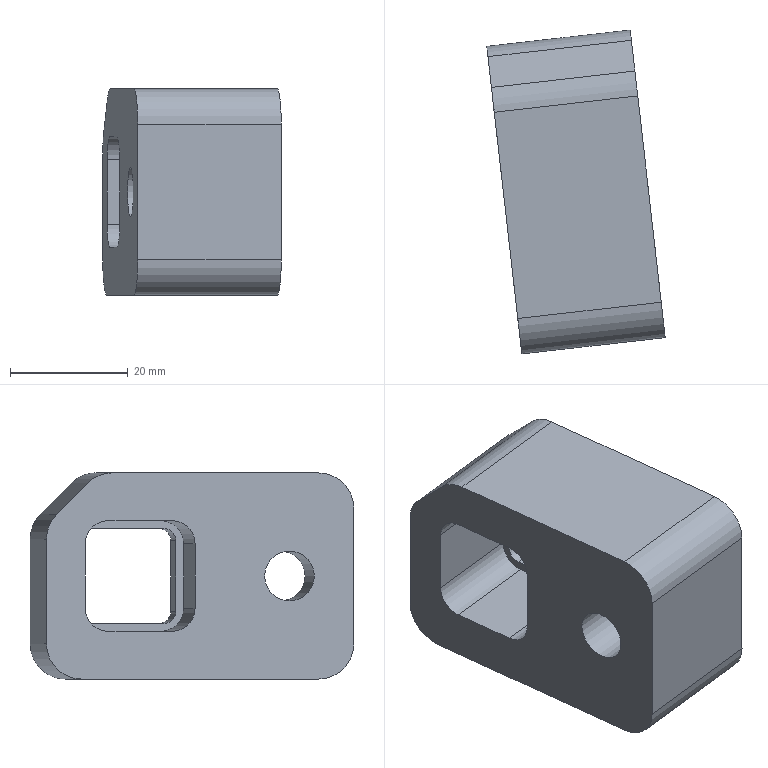Part | NX | features solid 2 | 1 solid | 32 faces | box 30.286 x 54.936 x 35 mm | volume 33387 mm3 | plane 17 | cylinder 15 | commonest cylinder face diameters 12 x5 4.08 x4 7.75 x4 8.5 x1 14 x1
STEP:
#1=CARTESIAN_POINT('',(3191.515,360.034,-76.987));
#2=VERTEX_POINT('',#1);
#3=CARTESIAN_POINT('',(3191.076,363.884,-80.862));
#4=VERTEX_POINT('',#3);
#5=CARTESIAN_POINT('',(3191.515,360.034,-80.862));
#6=DIRECTION('',(-0.9936,-0.1132,-0.000000001));
#7=DIRECTION('',(0.000000001,0.,-1.));
#8=AXIS2_PLACEMENT_3D('',#5,#6,#7);
#9=CIRCLE('',#8,3.875);
#10=EDGE_CURVE('',#2,#4,#9,.T.);
#11=ORIENTED_EDGE('',*,*,#10,.T.);
#12=CARTESIAN_POINT('',(3191.076,363.884,-91.862));
#13=VERTEX_POINT('',#12);
#14=CARTESIAN_POINT('',(3191.076,363.884,-86.362));
#15=DIRECTION('',(0.000000001,0.,-1.));
#16=VECTOR('',#15,1000.);
#17=LINE('',#14,#16);
#18=EDGE_CURVE('',#4,#13,#17,.T.);
#19=ORIENTED_EDGE('',*,*,#18,.T.);
#20=CARTESIAN_POINT('',(3191.515,360.034,-95.737));
#21=VERTEX_POINT('',#20);
#22=CARTESIAN_POINT('',(3191.515,360.034,-91.862));
#23=DIRECTION('',(-0.9936,-0.1132,-0.000000001));
#24=DIRECTION('',(0.000000001,0.,-1.));
#25=AXIS2_PLACEMENT_3D('',#22,#23,#24);
#26=CIRCLE('',#25,3.875);
#27=EDGE_CURVE('',#13,#21,#26,.T.);
#28=ORIENTED_EDGE('',*,*,#27,.T.);
#29=CARTESIAN_POINT('',(3192.76,349.105,-95.737));
#30=VERTEX_POINT('',#29);
#31=CARTESIAN_POINT('',(3192.222,353.824,-95.737));
#32=DIRECTION('',(0.1132,-0.9936,0.));
#33=VECTOR('',#32,1000.);
#34=LINE('',#31,#33);
#35=EDGE_CURVE('',#21,#30,#34,.T.);
#36=ORIENTED_EDGE('',*,*,#35,.T.);
#37=CARTESIAN_POINT('',(3193.198,345.255,-91.862));
#38=VERTEX_POINT('',#37);
#39=CARTESIAN_POINT('',(3192.76,349.105,-91.862));
#40=DIRECTION('',(0.9936,0.1132,0.000000001));
#41=DIRECTION('',(0.000000001,0.,-1.));
#42=AXIS2_PLACEMENT_3D('',#39,#40,#41);
#43=CIRCLE('',#42,3.875);
#44=EDGE_CURVE('',#38,#30,#43,.T.);
#45=ORIENTED_EDGE('',*,*,#44,.F.);
#46=CARTESIAN_POINT('',(3193.198,345.255,-80.862));
#47=VERTEX_POINT('',#46);
#48=CARTESIAN_POINT('',(3193.198,345.255,-91.862));
#49=DIRECTION('',(0.000000001,0.,-1.));
#50=VECTOR('',#49,1000.);
#51=LINE('',#48,#50);
#52=EDGE_CURVE('',#47,#38,#51,.T.);
#53=ORIENTED_EDGE('',*,*,#52,.F.);
#54=CARTESIAN_POINT('',(3192.76,349.105,-76.987));
#55=VERTEX_POINT('',#54);
#56=CARTESIAN_POINT('',(3192.76,349.105,-80.862));
#57=DIRECTION('',(0.9936,0.1132,0.000000001));
#58=DIRECTION('',(0.000000001,0.,-1.));
#59=AXIS2_PLACEMENT_3D('',#56,#57,#58);
#60=CIRCLE('',#59,3.875);
#61=EDGE_CURVE('',#55,#47,#60,.T.);
#62=ORIENTED_EDGE('',*,*,#61,.F.);
#63=CARTESIAN_POINT('',(3192.76,349.105,-76.987));
#64=DIRECTION('',(0.1132,-0.9936,0.));
#65=VECTOR('',#64,1000.);
#66=LINE('',#63,#65);
#67=EDGE_CURVE('',#2,#55,#66,.T.);
#68=ORIENTED_EDGE('',*,*,#67,.F.);
#69=EDGE_LOOP('',(#11,#19,#28,#36,#45,#53,#62,#68));
#70=FACE_BOUND('',#69,.T.);
#71=CARTESIAN_POINT('',(3193.047,346.581,-80.362));
#72=VERTEX_POINT('',#71);
#73=CARTESIAN_POINT('',(3193.047,346.581,-92.362));
#74=VERTEX_POINT('',#73);
#75=CARTESIAN_POINT('',(3193.047,346.581,-86.362));
#76=DIRECTION('',(0.000000001,-0.000000001,-1.));
#77=VECTOR('',#76,1000.);
#78=LINE('',#75,#77);
#79=EDGE_CURVE('',#72,#74,#78,.T.);
#80=ORIENTED_EDGE('',*,*,#79,.T.);
#81=CARTESIAN_POINT('',(3192.816,348.608,-94.402));
#82=VERTEX_POINT('',#81);
#83=CARTESIAN_POINT('',(3192.816,348.608,-92.362));
#84=DIRECTION('',(0.9936,0.1132,0.000000001));
#85=DIRECTION('',(0.000000001,0.,-1.));
#86=AXIS2_PLACEMENT_3D('',#83,#84,#85);
#87=CIRCLE('',#86,2.04);
#88=EDGE_CURVE('',#74,#82,#87,.T.);
#89=ORIENTED_EDGE('',*,*,#88,.T.);
#90=CARTESIAN_POINT('',(3191.458,360.531,-94.402));
#91=VERTEX_POINT('',#90);
#92=CARTESIAN_POINT('',(3192.222,353.824,-94.402));
#93=DIRECTION('',(-0.1132,0.9936,-0.000000001));
#94=VECTOR('',#93,1000.);
#95=LINE('',#92,#94);
#96=EDGE_CURVE('',#82,#91,#95,.T.);
#97=ORIENTED_EDGE('',*,*,#96,.T.);
#98=CARTESIAN_POINT('',(3191.227,362.558,-92.362));
#99=VERTEX_POINT('',#98);
#100=CARTESIAN_POINT('',(3191.458,360.531,-92.362));
#101=DIRECTION('',(0.9936,0.1132,0.000000001));
#102=DIRECTION('',(0.000000001,0.,-1.));
#103=AXIS2_PLACEMENT_3D('',#100,#101,#102);
#104=CIRCLE('',#103,2.04);
#105=EDGE_CURVE('',#91,#99,#104,.T.);
#106=ORIENTED_EDGE('',*,*,#105,.T.);
#107=CARTESIAN_POINT('',(3191.227,362.558,-80.362));
#108=VERTEX_POINT('',#107);
#109=CARTESIAN_POINT('',(3191.227,362.558,-86.362));
#110=DIRECTION('',(-0.000000001,0.000000001,1.));
#111=VECTOR('',#110,1000.);
#112=LINE('',#109,#111);
#113=EDGE_CURVE('',#99,#108,#112,.T.);
#114=ORIENTED_EDGE('',*,*,#113,.T.);
#115=CARTESIAN_POINT('',(3191.458,360.531,-78.322));
#116=VERTEX_POINT('',#115);
#117=CARTESIAN_POINT('',(3191.458,360.531,-80.362));
#118=DIRECTION('',(0.9936,0.1132,0.000000001));
#119=DIRECTION('',(0.000000001,0.,-1.));
#120=AXIS2_PLACEMENT_3D('',#117,#118,#119);
#121=CIRCLE('',#120,2.04);
#122=EDGE_CURVE('',#108,#116,#121,.T.);
#123=ORIENTED_EDGE('',*,*,#122,.T.);
#124=CARTESIAN_POINT('',(3192.816,348.608,-78.322));
#125=VERTEX_POINT('',#124);
#126=CARTESIAN_POINT('',(3192.222,353.824,-78.322));
#127=DIRECTION('',(0.1132,-0.9936,0.));
#128=VECTOR('',#127,1000.);
#129=LINE('',#126,#128);
#130=EDGE_CURVE('',#116,#125,#129,.T.);
#131=ORIENTED_EDGE('',*,*,#130,.T.);
#132=CARTESIAN_POINT('',(3192.816,348.608,-80.362));
#133=DIRECTION('',(0.9936,0.1132,0.000000001));
#134=DIRECTION('',(0.000000001,0.,-1.));
#135=AXIS2_PLACEMENT_3D('',#132,#133,#134);
#136=CIRCLE('',#135,2.04);
#137=EDGE_CURVE('',#125,#72,#136,.T.);
#138=ORIENTED_EDGE('',*,*,#137,.T.);
#139=EDGE_LOOP('',(#80,#89,#97,#106,#114,#123,#131,#138));
#140=FACE_BOUND('',#139,.T.);
#141=CARTESIAN_POINT('',(3192.222,353.824,-86.362));
#142=DIRECTION('',(-0.9936,-0.1132,-0.000000001));
#143=DIRECTION('',(0.000000001,0.,-1.));
#144=AXIS2_PLACEMENT_3D('',#141,#142,#143);
#145=PLANE('',#144);
#146=ADVANCED_FACE('',(#70,#140),#145,.T.);
#147=CARTESIAN_POINT('',(3197.778,371.316,-80.13));
#148=VERTEX_POINT('',#147);
#149=CARTESIAN_POINT('',(3197.778,371.316,-97.862));
#150=VERTEX_POINT('',#149);
#151=CARTESIAN_POINT('',(3197.778,371.316,-86.362));
#152=DIRECTION('',(0.000000001,0.,-1.));
#153=VECTOR('',#152,1000.);
#154=LINE('',#151,#153);
#155=EDGE_CURVE('',#148,#150,#154,.T.);
#156=ORIENTED_EDGE('',*,*,#155,.F.);
#157=CARTESIAN_POINT('',(3197.977,369.569,-75.887));
#158=VERTEX_POINT('',#157);
#159=CARTESIAN_POINT('',(3198.457,365.354,-80.13));
#160=DIRECTION('',(-0.9936,-0.1132,-0.000000001));
#161=DIRECTION('',(-0.000000001,0.,1.));
#162=AXIS2_PLACEMENT_3D('',#159,#160,#161);
#163=CIRCLE('',#162,6.);
#164=EDGE_CURVE('',#158,#148,#163,.T.);
#165=ORIENTED_EDGE('',*,*,#164,.F.);
#166=CARTESIAN_POINT('',(3198.573,364.335,-70.619));
#167=VERTEX_POINT('',#166);
#168=CARTESIAN_POINT('',(3200.143,350.558,-56.753));
#169=DIRECTION('',(-0.08005,0.7026,-0.7071));
#170=VECTOR('',#169,1000.);
#171=LINE('',#168,#170);
#172=EDGE_CURVE('',#167,#158,#171,.T.);
#173=ORIENTED_EDGE('',*,*,#172,.F.);
#174=CARTESIAN_POINT('',(3199.053,360.12,-68.862));
#175=VERTEX_POINT('',#174);
#176=CARTESIAN_POINT('',(3199.053,360.12,-74.862));
#177=DIRECTION('',(-0.9936,-0.1132,-0.000000001));
#178=DIRECTION('',(-0.000000001,0.,1.));
#179=AXIS2_PLACEMENT_3D('',#176,#177,#178);
#180=CIRCLE('',#179,6.);
#181=EDGE_CURVE('',#175,#167,#180,.T.);
#182=ORIENTED_EDGE('',*,*,#181,.F.);
#183=CARTESIAN_POINT('',(3203.042,325.114,-68.862));
#184=VERTEX_POINT('',#183);
#185=CARTESIAN_POINT('',(3203.494,321.14,-68.862));
#186=DIRECTION('',(-0.1132,0.9936,0.));
#187=VECTOR('',#186,1000.);
#188=LINE('',#185,#187);
#189=EDGE_CURVE('',#184,#175,#188,.T.);
#190=ORIENTED_EDGE('',*,*,#189,.F.);
#191=CARTESIAN_POINT('',(3203.721,319.153,-74.862));
#192=VERTEX_POINT('',#191);
#193=CARTESIAN_POINT('',(3203.042,325.114,-74.862));
#194=DIRECTION('',(-0.9936,-0.1132,-0.000000001));
#195=DIRECTION('',(-0.000000001,0.,1.));
#196=AXIS2_PLACEMENT_3D('',#193,#194,#195);
#197=CIRCLE('',#196,6.);
#198=EDGE_CURVE('',#192,#184,#197,.T.);
#199=ORIENTED_EDGE('',*,*,#198,.F.);
#200=CARTESIAN_POINT('',(3203.721,319.153,-97.862));
#201=VERTEX_POINT('',#200);
#202=CARTESIAN_POINT('',(3203.721,319.153,-86.362));
#203=DIRECTION('',(-0.000000001,0.,1.));
#204=VECTOR('',#203,1000.);
#205=LINE('',#202,#204);
#206=EDGE_CURVE('',#201,#192,#205,.T.);
#207=ORIENTED_EDGE('',*,*,#206,.F.);
#208=CARTESIAN_POINT('',(3203.042,325.114,-103.862));
#209=VERTEX_POINT('',#208);
#210=CARTESIAN_POINT('',(3203.042,325.114,-97.862));
#211=DIRECTION('',(-0.9936,-0.1132,-0.000000001));
#212=DIRECTION('',(-0.000000001,0.,1.));
#213=AXIS2_PLACEMENT_3D('',#210,#211,#212);
#214=CIRCLE('',#213,6.);
#215=EDGE_CURVE('',#209,#201,#214,.T.);
#216=ORIENTED_EDGE('',*,*,#215,.F.);
#217=CARTESIAN_POINT('',(3198.457,365.354,-103.862));
#218=VERTEX_POINT('',#217);
#219=CARTESIAN_POINT('',(3203.494,321.14,-103.862));
#220=DIRECTION('',(-0.1132,0.9936,0.));
#221=VECTOR('',#220,1000.);
#222=LINE('',#219,#221);
#223=EDGE_CURVE('',#209,#218,#222,.T.);
#224=ORIENTED_EDGE('',*,*,#223,.T.);
#225=CARTESIAN_POINT('',(3198.457,365.354,-97.862));
#226=DIRECTION('',(-0.9936,-0.1132,-0.000000001));
#227=DIRECTION('',(-0.000000001,0.,1.));
#228=AXIS2_PLACEMENT_3D('',#225,#226,#227);
#229=CIRCLE('',#228,6.);
#230=EDGE_CURVE('',#150,#218,#229,.T.);
#231=ORIENTED_EDGE('',*,*,#230,.F.);
#232=EDGE_LOOP('',(#156,#165,#173,#182,#190,#199,#207,#216,#224,#231));
#233=FACE_BOUND('',#232,.T.);
#234=CARTESIAN_POINT('',(3202.476,330.082,-79.362));
#235=VERTEX_POINT('',#234);
#236=CARTESIAN_POINT('',(3202.476,330.082,-86.362));
#237=DIRECTION('',(0.9936,0.1132,0.000000001));
#238=DIRECTION('',(-0.000000001,0.,1.));
#239=AXIS2_PLACEMENT_3D('',#236,#237,#238);
#240=CIRCLE('',#239,7.);
#241=EDGE_CURVE('',#235,#235,#240,.T.);
#242=ORIENTED_EDGE('',*,*,#241,.F.);
#243=EDGE_LOOP('',(#242));
#244=FACE_BOUND('',#243,.T.);
#245=CARTESIAN_POINT('',(3198.91,361.38,-78.322));
#246=VERTEX_POINT('',#245);
#247=CARTESIAN_POINT('',(3198.679,363.407,-80.362));
#248=VERTEX_POINT('',#247);
#249=CARTESIAN_POINT('',(3198.91,361.38,-80.362));
#250=DIRECTION('',(-0.9936,-0.1132,-0.000000001));
#251=DIRECTION('',(-0.000000001,0.,1.));
#252=AXIS2_PLACEMENT_3D('',#249,#250,#251);
#253=CIRCLE('',#252,2.04);
#254=EDGE_CURVE('',#246,#248,#253,.T.);
#255=ORIENTED_EDGE('',*,*,#254,.T.);
#256=CARTESIAN_POINT('',(3198.679,363.407,-92.362));
#257=VERTEX_POINT('',#256);
#258=CARTESIAN_POINT('',(3198.679,363.407,-86.362));
#259=DIRECTION('',(-0.000000001,0.000000001,1.));
#260=VECTOR('',#259,1000.);
#261=LINE('',#258,#260);
#262=EDGE_CURVE('',#257,#248,#261,.T.);
#263=ORIENTED_EDGE('',*,*,#262,.F.);
#264=CARTESIAN_POINT('',(3198.91,361.38,-94.402));
#265=VERTEX_POINT('',#264);
#266=CARTESIAN_POINT('',(3198.91,361.38,-92.362));
#267=DIRECTION('',(-0.9936,-0.1132,-0.000000001));
#268=DIRECTION('',(-0.000000001,0.,1.));
#269=AXIS2_PLACEMENT_3D('',#266,#267,#268);
#270=CIRCLE('',#269,2.04);
#271=EDGE_CURVE('',#257,#265,#270,.T.);
#272=ORIENTED_EDGE('',*,*,#271,.T.);
#273=CARTESIAN_POINT('',(3200.268,349.457,-94.402));
#274=VERTEX_POINT('',#273);
#275=CARTESIAN_POINT('',(3203.494,321.14,-94.402));
#276=DIRECTION('',(-0.1132,0.9936,-0.000000001));
#277=VECTOR('',#276,1000.);
#278=LINE('',#275,#277);
#279=EDGE_CURVE('',#274,#265,#278,.T.);
#280=ORIENTED_EDGE('',*,*,#279,.F.);
#281=CARTESIAN_POINT('',(3200.499,347.43,-92.362));
#282=VERTEX_POINT('',#281);
#283=CARTESIAN_POINT('',(3200.268,349.457,-92.362));
#284=DIRECTION('',(-0.9936,-0.1132,-0.000000001));
#285=DIRECTION('',(-0.000000001,0.,1.));
#286=AXIS2_PLACEMENT_3D('',#283,#284,#285);
#287=CIRCLE('',#286,2.04);
#288=EDGE_CURVE('',#274,#282,#287,.T.);
#289=ORIENTED_EDGE('',*,*,#288,.T.);
#290=CARTESIAN_POINT('',(3200.499,347.43,-80.362));
#291=VERTEX_POINT('',#290);
#292=CARTESIAN_POINT('',(3200.499,347.43,-86.362));
#293=DIRECTION('',(0.000000001,-0.000000001,-1.));
#294=VECTOR('',#293,1000.);
#295=LINE('',#292,#294);
#296=EDGE_CURVE('',#291,#282,#295,.T.);
#297=ORIENTED_EDGE('',*,*,#296,.F.);
#298=CARTESIAN_POINT('',(3200.268,349.457,-78.322));
#299=VERTEX_POINT('',#298);
#300=CARTESIAN_POINT('',(3200.268,349.457,-80.362));
#301=DIRECTION('',(-0.9936,-0.1132,-0.000000001));
#302=DIRECTION('',(-0.000000001,0.,1.));
#303=AXIS2_PLACEMENT_3D('',#300,#301,#302);
#304=CIRCLE('',#303,2.04);
#305=EDGE_CURVE('',#291,#299,#304,.T.);
#306=ORIENTED_EDGE('',*,*,#305,.T.);
#307=CARTESIAN_POINT('',(3203.494,321.14,-78.322));
#308=DIRECTION('',(0.1132,-0.9936,0.));
#309=VECTOR('',#308,1000.);
#310=LINE('',#307,#309);
#311=EDGE_CURVE('',#246,#299,#310,.T.);
#312=ORIENTED_EDGE('',*,*,#311,.F.);
#313=EDGE_LOOP('',(#255,#263,#272,#280,#289,#297,#306,#312));
#314=FACE_BOUND('',#313,.T.);
#315=CARTESIAN_POINT('',(3203.494,321.14,-86.362));
#316=DIRECTION('',(0.9936,0.1132,0.000000001));
#317=DIRECTION('',(0.1132,-0.9936,0.));
#318=AXIS2_PLACEMENT_3D('',#315,#316,#317);
#319=PLANE('',#318);
#320=ADVANCED_FACE('',(#233,#244,#314),#319,.T.);
#321=CARTESIAN_POINT('',(3178.699,322.341,-103.862));
#322=VERTEX_POINT('',#321);
#323=CARTESIAN_POINT('',(3174.114,362.581,-103.862));
#324=VERTEX_POINT('',#323);
#325=CARTESIAN_POINT('',(3179.152,318.367,-103.862));
#326=DIRECTION('',(-0.1132,0.9936,0.));
#327=VECTOR('',#326,1000.);
#328=LINE('',#325,#327);
#329=EDGE_CURVE('',#322,#324,#328,.T.);
#330=ORIENTED_EDGE('',*,*,#329,.F.);
#331=CARTESIAN_POINT('',(3179.378,316.38,-97.862));
#332=VERTEX_POINT('',#331);
#333=CARTESIAN_POINT('',(3178.699,322.341,-97.862));
#334=DIRECTION('',(0.9936,0.1132,0.000000001));
#335=DIRECTION('',(-0.1132,0.9936,0.));
#336=AXIS2_PLACEMENT_3D('',#333,#334,#335);
#337=CIRCLE('',#336,6.);
#338=EDGE_CURVE('',#332,#322,#337,.T.);
#339=ORIENTED_EDGE('',*,*,#338,.F.);
#340=CARTESIAN_POINT('',(3179.378,316.38,-74.862));
#341=VERTEX_POINT('',#340);
#342=CARTESIAN_POINT('',(3179.378,316.38,-86.362));
#343=DIRECTION('',(0.000000001,0.,-1.));
#344=VECTOR('',#343,1000.);
#345=LINE('',#342,#344);
#346=EDGE_CURVE('',#341,#332,#345,.T.);
#347=ORIENTED_EDGE('',*,*,#346,.F.);
#348=CARTESIAN_POINT('',(3178.699,322.341,-68.862));
#349=VERTEX_POINT('',#348);
#350=CARTESIAN_POINT('',(3178.699,322.341,-74.862));
#351=DIRECTION('',(0.9936,0.1132,0.000000001));
#352=DIRECTION('',(-0.1132,0.9936,0.));
#353=AXIS2_PLACEMENT_3D('',#350,#351,#352);
#354=CIRCLE('',#353,6.);
#355=EDGE_CURVE('',#349,#341,#354,.T.);
#356=ORIENTED_EDGE('',*,*,#355,.F.);
#357=CARTESIAN_POINT('',(3174.711,357.346,-68.862));
#358=VERTEX_POINT('',#357);
#359=CARTESIAN_POINT('',(3179.152,318.367,-68.862));
#360=DIRECTION('',(-0.1132,0.9936,0.));
#361=VECTOR('',#360,1000.);
#362=LINE('',#359,#361);
#363=EDGE_CURVE('',#349,#358,#362,.T.);
#364=ORIENTED_EDGE('',*,*,#363,.T.);
#365=CARTESIAN_POINT('',(3174.23,361.562,-70.619));
#366=VERTEX_POINT('',#365);
#367=CARTESIAN_POINT('',(3174.711,357.346,-74.862));
#368=DIRECTION('',(0.9936,0.1132,0.000000001));
#369=DIRECTION('',(-0.1132,0.9936,0.));
#370=AXIS2_PLACEMENT_3D('',#367,#368,#369);
#371=CIRCLE('',#370,6.);
#372=EDGE_CURVE('',#366,#358,#371,.T.);
#373=ORIENTED_EDGE('',*,*,#372,.F.);
#374=CARTESIAN_POINT('',(3173.634,366.796,-75.887));
#375=VERTEX_POINT('',#374);
#376=CARTESIAN_POINT('',(3175.8,347.785,-56.753));
#377=DIRECTION('',(0.08005,-0.7026,0.7071));
#378=VECTOR('',#377,1000.);
#379=LINE('',#376,#378);
#380=EDGE_CURVE('',#375,#366,#379,.T.);
#381=ORIENTED_EDGE('',*,*,#380,.F.);
#382=CARTESIAN_POINT('',(3173.435,368.542,-80.13));
#383=VERTEX_POINT('',#382);
#384=CARTESIAN_POINT('',(3174.114,362.581,-80.13));
#385=DIRECTION('',(0.9936,0.1132,0.000000001));
#386=DIRECTION('',(-0.1132,0.9936,0.));
#387=AXIS2_PLACEMENT_3D('',#384,#385,#386);
#388=CIRCLE('',#387,6.);
#389=EDGE_CURVE('',#383,#375,#388,.T.);
#390=ORIENTED_EDGE('',*,*,#389,.F.);
#391=CARTESIAN_POINT('',(3173.435,368.542,-97.862));
#392=VERTEX_POINT('',#391);
#393=CARTESIAN_POINT('',(3173.435,368.542,-86.362));
#394=DIRECTION('',(-0.000000001,0.,1.));
#395=VECTOR('',#394,1000.);
#396=LINE('',#393,#395);
#397=EDGE_CURVE('',#392,#383,#396,.T.);
#398=ORIENTED_EDGE('',*,*,#397,.F.);
#399=CARTESIAN_POINT('',(3174.114,362.581,-97.862));
#400=DIRECTION('',(0.9936,0.1132,0.000000001));
#401=DIRECTION('',(-0.1132,0.9936,0.));
#402=AXIS2_PLACEMENT_3D('',#399,#400,#401);
#403=CIRCLE('',#402,6.);
#404=EDGE_CURVE('',#324,#392,#403,.T.);
#405=ORIENTED_EDGE('',*,*,#404,.F.);
#406=EDGE_LOOP('',(#330,#339,#347,#356,#364,#373,#381,#390,#398,#405));
#407=FACE_BOUND('',#406,.T.);
#408=CARTESIAN_POINT('',(3177.652,331.531,-86.362));
#409=VERTEX_POINT('',#408);
#410=CARTESIAN_POINT('',(3178.133,327.309,-86.362));
#411=DIRECTION('',(0.9936,0.1132,0.000000001));
#412=DIRECTION('',(-0.1132,0.9936,0.));
#413=AXIS2_PLACEMENT_3D('',#410,#411,#412);
#414=CIRCLE('',#413,4.25);
#415=EDGE_CURVE('',#409,#409,#414,.T.);
#416=ORIENTED_EDGE('',*,*,#415,.T.);
#417=EDGE_LOOP('',(#416));
#418=FACE_BOUND('',#417,.T.);
#419=CARTESIAN_POINT('',(3174.185,361.96,-80.862));
#420=VERTEX_POINT('',#419);
#421=CARTESIAN_POINT('',(3174.624,358.11,-76.987));
#422=VERTEX_POINT('',#421);
#423=CARTESIAN_POINT('',(3174.624,358.11,-80.862));
#424=DIRECTION('',(0.9936,0.1132,0.000000001));
#425=DIRECTION('',(-0.1132,0.9936,0.));
#426=AXIS2_PLACEMENT_3D('',#423,#424,#425);
#427=CIRCLE('',#426,3.875);
#428=EDGE_CURVE('',#420,#422,#427,.T.);
#429=ORIENTED_EDGE('',*,*,#428,.T.);
#430=CARTESIAN_POINT('',(3175.869,347.18,-76.987));
#431=VERTEX_POINT('',#430);
#432=CARTESIAN_POINT('',(3179.152,318.367,-76.987));
#433=DIRECTION('',(-0.1132,0.9936,0.));
#434=VECTOR('',#433,1000.);
#435=LINE('',#432,#434);
#436=EDGE_CURVE('',#431,#422,#435,.T.);
#437=ORIENTED_EDGE('',*,*,#436,.F.);
#438=CARTESIAN_POINT('',(3176.308,343.33,-80.862));
#439=VERTEX_POINT('',#438);
#440=CARTESIAN_POINT('',(3175.869,347.18,-80.862));
#441=DIRECTION('',(0.9936,0.1132,0.000000001));
#442=DIRECTION('',(-0.1132,0.9936,0.));
#443=AXIS2_PLACEMENT_3D('',#440,#441,#442);
#444=CIRCLE('',#443,3.875);
#445=EDGE_CURVE('',#431,#439,#444,.T.);
#446=ORIENTED_EDGE('',*,*,#445,.T.);
#447=CARTESIAN_POINT('',(3176.308,343.33,-91.862));
#448=VERTEX_POINT('',#447);
#449=CARTESIAN_POINT('',(3176.308,343.33,-86.362));
#450=DIRECTION('',(-0.000000001,0.,1.));
#451=VECTOR('',#450,1000.);
#452=LINE('',#449,#451);
#453=EDGE_CURVE('',#448,#439,#452,.T.);
#454=ORIENTED_EDGE('',*,*,#453,.F.);
#455=CARTESIAN_POINT('',(3175.869,347.18,-95.737));
#456=VERTEX_POINT('',#455);
#457=CARTESIAN_POINT('',(3175.869,347.18,-91.862));
#458=DIRECTION('',(0.9936,0.1132,0.000000001));
#459=DIRECTION('',(-0.1132,0.9936,0.));
#460=AXIS2_PLACEMENT_3D('',#457,#458,#459);
#461=CIRCLE('',#460,3.875);
#462=EDGE_CURVE('',#448,#456,#461,.T.);
#463=ORIENTED_EDGE('',*,*,#462,.T.);
#464=CARTESIAN_POINT('',(3174.624,358.11,-95.737));
#465=VERTEX_POINT('',#464);
#466=CARTESIAN_POINT('',(3179.152,318.367,-95.737));
#467=DIRECTION('',(0.1132,-0.9936,0.));
#468=VECTOR('',#467,1000.);
#469=LINE('',#466,#468);
#470=EDGE_CURVE('',#465,#456,#469,.T.);
#471=ORIENTED_EDGE('',*,*,#470,.F.);
#472=CARTESIAN_POINT('',(3174.185,361.96,-91.862));
#473=VERTEX_POINT('',#472);
#474=CARTESIAN_POINT('',(3174.624,358.11,-91.862));
#475=DIRECTION('',(0.9936,0.1132,0.000000001));
#476=DIRECTION('',(-0.1132,0.9936,0.));
#477=AXIS2_PLACEMENT_3D('',#474,#475,#476);
#478=CIRCLE('',#477,3.875);
#479=EDGE_CURVE('',#465,#473,#478,.T.);
#480=ORIENTED_EDGE('',*,*,#479,.T.);
#481=CARTESIAN_POINT('',(3174.185,361.96,-86.362));
#482=DIRECTION('',(0.000000001,0.,-1.));
#483=VECTOR('',#482,1000.);
#484=LINE('',#481,#483);
#485=EDGE_CURVE('',#420,#473,#484,.T.);
#486=ORIENTED_EDGE('',*,*,#485,.F.);
#487=EDGE_LOOP('',(#429,#437,#446,#454,#463,#471,#480,#486));
#488=FACE_BOUND('',#487,.T.);
#489=CARTESIAN_POINT('',(3179.152,318.367,-86.362));
#490=DIRECTION('',(-0.9936,-0.1132,-0.000000001));
#491=DIRECTION('',(-0.1132,0.9936,0.));
#492=AXIS2_PLACEMENT_3D('',#489,#490,#491);
#493=PLANE('',#492);
#494=ADVANCED_FACE('',(#407,#418,#488),#493,.T.);
#495=ORIENTED_EDGE('',*,*,#415,.F.);
#496=EDGE_LOOP('',(#495));
#497=FACE_BOUND('',#496,.T.);
#498=CARTESIAN_POINT('',(3192.524,324.671,-86.362));
#499=VERTEX_POINT('',#498);
#500=CARTESIAN_POINT('',(3192.043,328.894,-86.362));
#501=DIRECTION('',(0.9936,0.1132,0.000000001));
#502=DIRECTION('',(0.1132,-0.9936,0.));
#503=AXIS2_PLACEMENT_3D('',#500,#501,#502);
#504=CIRCLE('',#503,4.25);
#505=EDGE_CURVE('',#499,#499,#504,.T.);
#506=ORIENTED_EDGE('',*,*,#505,.T.);
#507=EDGE_LOOP('',(#506));
#508=FACE_BOUND('',#507,.T.);
#509=CARTESIAN_POINT('',(3237.747,334.101,-86.362));
#510=DIRECTION('',(-0.9936,-0.1132,-0.000000001));
#511=DIRECTION('',(0.000000001,0.,-1.));
#512=AXIS2_PLACEMENT_3D('',#509,#510,#511);
#513=CYLINDRICAL_SURFACE('',#512,4.25);
#514=ADVANCED_FACE('',(#497,#508),#513,.F.);
#515=ORIENTED_EDGE('',*,*,#397,.T.);
#516=CARTESIAN_POINT('',(3185.855,369.957,-80.13));
#517=DIRECTION('',(-0.9936,-0.1132,-0.000000001));
#518=VECTOR('',#517,1000.);
#519=LINE('',#516,#518);
#520=EDGE_CURVE('',#148,#383,#519,.T.);
#521=ORIENTED_EDGE('',*,*,#520,.F.);
#522=ORIENTED_EDGE('',*,*,#155,.T.);
#523=CARTESIAN_POINT('',(3185.855,369.957,-97.862));
#524=DIRECTION('',(0.9936,0.1132,0.000000001));
#525=VECTOR('',#524,1000.);
#526=LINE('',#523,#525);
#527=EDGE_CURVE('',#392,#150,#526,.T.);
#528=ORIENTED_EDGE('',*,*,#527,.F.);
#529=EDGE_LOOP('',(#515,#521,#522,#528));
#530=FACE_BOUND('',#529,.T.);
#531=CARTESIAN_POINT('',(3185.855,369.957,-86.362));
#532=DIRECTION('',(-0.1132,0.9936,0.));
#533=DIRECTION('',(0.9936,0.1132,0.000000001));
#534=AXIS2_PLACEMENT_3D('',#531,#532,#533);
#535=PLANE('',#534);
#536=ADVANCED_FACE('',(#530),#535,.T.);
#537=ORIENTED_EDGE('',*,*,#223,.F.);
#538=CARTESIAN_POINT('',(3191.119,323.756,-103.862));
#539=DIRECTION('',(0.9936,0.1132,0.000000001));
#540=VECTOR('',#539,1000.);
#541=LINE('',#538,#540);
#542=EDGE_CURVE('',#322,#209,#541,.T.);
#543=ORIENTED_EDGE('',*,*,#542,.F.);
#544=ORIENTED_EDGE('',*,*,#329,.T.);
#545=CARTESIAN_POINT('',(3186.534,363.996,-103.862));
#546=DIRECTION('',(-0.9936,-0.1132,-0.000000001));
#547=VECTOR('',#546,1000.);
#548=LINE('',#545,#547);
#549=EDGE_CURVE('',#218,#324,#548,.T.);
#550=ORIENTED_EDGE('',*,*,#549,.F.);
#551=EDGE_LOOP('',(#537,#543,#544,#550));
#552=FACE_BOUND('',#551,.T.);
#553=CARTESIAN_POINT('',(3191.572,319.782,-103.862));
#554=DIRECTION('',(0.000000001,0.,-1.));
#555=DIRECTION('',(0.1132,-0.9936,0.));
#556=AXIS2_PLACEMENT_3D('',#553,#554,#555);
#557=PLANE('',#556);
#558=ADVANCED_FACE('',(#552),#557,.T.);
#559=ORIENTED_EDGE('',*,*,#189,.T.);
#560=CARTESIAN_POINT('',(3187.13,358.761,-68.862));
#561=DIRECTION('',(0.9936,0.1132,0.000000001));
#562=VECTOR('',#561,1000.);
#563=LINE('',#560,#562);
#564=EDGE_CURVE('',#358,#175,#563,.T.);
#565=ORIENTED_EDGE('',*,*,#564,.F.);
#566=ORIENTED_EDGE('',*,*,#363,.F.);
#567=CARTESIAN_POINT('',(3191.119,323.756,-68.862));
#568=DIRECTION('',(-0.9936,-0.1132,-0.000000001));
#569=VECTOR('',#568,1000.);
#570=LINE('',#567,#569);
#571=EDGE_CURVE('',#184,#349,#570,.T.);
#572=ORIENTED_EDGE('',*,*,#571,.F.);
#573=EDGE_LOOP('',(#559,#565,#566,#572));
#574=FACE_BOUND('',#573,.T.);
#575=CARTESIAN_POINT('',(3191.572,319.782,-68.862));
#576=DIRECTION('',(-0.000000001,0.,1.));
#577=DIRECTION('',(-0.1132,0.9936,0.));
#578=AXIS2_PLACEMENT_3D('',#575,#576,#577);
#579=PLANE('',#578);
#580=ADVANCED_FACE('',(#574),#579,.T.);
#581=ORIENTED_EDGE('',*,*,#346,.T.);
#582=CARTESIAN_POINT('',(3191.798,317.795,-97.862));
#583=DIRECTION('',(-0.9936,-0.1132,-0.000000001));
#584=VECTOR('',#583,1000.);
#585=LINE('',#582,#584);
#586=EDGE_CURVE('',#201,#332,#585,.T.);
#587=ORIENTED_EDGE('',*,*,#586,.F.);
#588=ORIENTED_EDGE('',*,*,#206,.T.);
#589=CARTESIAN_POINT('',(3191.798,317.795,-74.862));
#590=DIRECTION('',(0.9936,0.1132,0.000000001));
#591=VECTOR('',#590,1000.);
#592=LINE('',#589,#591);
#593=EDGE_CURVE('',#341,#192,#592,.T.);
#594=ORIENTED_EDGE('',*,*,#593,.F.);
#595=EDGE_LOOP('',(#581,#587,#588,#594));
#596=FACE_BOUND('',#595,.T.);
#597=CARTESIAN_POINT('',(3191.798,317.795,-86.362));
#598=DIRECTION('',(0.1132,-0.9936,0.));
#599=DIRECTION('',(-0.9936,-0.1132,-0.000000001));
#600=AXIS2_PLACEMENT_3D('',#597,#598,#599);
#601=PLANE('',#600);
#602=ADVANCED_FACE('',(#596),#601,.T.);
#603=ORIENTED_EDGE('',*,*,#172,.T.);
#604=CARTESIAN_POINT('',(3186.054,368.211,-75.887));
#605=DIRECTION('',(0.9936,0.1132,0.000000001));
#606=VECTOR('',#605,1000.);
#607=LINE('',#604,#606);
#608=EDGE_CURVE('',#375,#158,#607,.T.);
#609=ORIENTED_EDGE('',*,*,#608,.F.);
#610=ORIENTED_EDGE('',*,*,#380,.T.);
#611=CARTESIAN_POINT('',(3186.65,362.977,-70.619));
#612=DIRECTION('',(-0.9936,-0.1132,-0.000000001));
#613=VECTOR('',#612,1000.);
#614=LINE('',#611,#613);
#615=EDGE_CURVE('',#167,#366,#614,.T.);
#616=ORIENTED_EDGE('',*,*,#615,.F.);
#617=EDGE_LOOP('',(#603,#609,#610,#616));
#618=FACE_BOUND('',#617,.T.);
#619=CARTESIAN_POINT('',(3186.833,361.371,-69.003));
#620=DIRECTION('',(0.08005,-0.7026,-0.7071));
#621=DIRECTION('',(0.9936,0.1132,0.000000001));
#622=AXIS2_PLACEMENT_3D('',#619,#620,#621);
#623=PLANE('',#622);
#624=ADVANCED_FACE('',(#618),#623,.F.);
#625=CARTESIAN_POINT('',(3192.043,328.894,-79.362));
#626=VERTEX_POINT('',#625);
#627=CARTESIAN_POINT('',(3192.043,328.894,-86.362));
#628=DIRECTION('',(0.9936,0.1132,0.000000001));
#629=DIRECTION('',(-0.000000001,0.,1.));
#630=AXIS2_PLACEMENT_3D('',#627,#628,#629);
#631=CIRCLE('',#630,7.);
#632=EDGE_CURVE('',#626,#626,#631,.T.);
#633=ORIENTED_EDGE('',*,*,#632,.T.);
#634=EDGE_LOOP('',(#633));
#635=FACE_BOUND('',#634,.T.);
#636=ORIENTED_EDGE('',*,*,#505,.F.);
#637=EDGE_LOOP('',(#636));
#638=FACE_BOUND('',#637,.T.);
#639=CARTESIAN_POINT('',(3192.043,328.894,-86.362));
#640=DIRECTION('',(0.9936,0.1132,0.000000001));
#641=DIRECTION('',(0.1132,-0.9936,0.));
#642=AXIS2_PLACEMENT_3D('',#639,#640,#641);
#643=PLANE('',#642);
#644=ADVANCED_FACE('',(#635,#638),#643,.T.);
#645=ORIENTED_EDGE('',*,*,#241,.T.);
#646=EDGE_LOOP('',(#645));
#647=FACE_BOUND('',#646,.T.);
#648=ORIENTED_EDGE('',*,*,#632,.F.);
#649=EDGE_LOOP('',(#648));
#650=FACE_BOUND('',#649,.T.);
#651=CARTESIAN_POINT('',(3213.902,331.384,-86.362));
#652=DIRECTION('',(-0.9936,-0.1132,-0.000000001));
#653=DIRECTION('',(-0.1132,0.9936,0.));
#654=AXIS2_PLACEMENT_3D('',#651,#652,#653);
#655=CYLINDRICAL_SURFACE('',#654,7.);
#656=ADVANCED_FACE('',(#647,#650),#655,.F.);
#657=CARTESIAN_POINT('',(3285.162,359.633,-76.987));
#658=DIRECTION('',(0.9936,0.1132,0.000000001));
#659=VECTOR('',#658,1000.);
#660=LINE('',#657,#659);
#661=EDGE_CURVE('',#431,#55,#660,.T.);
#662=ORIENTED_EDGE('',*,*,#661,.F.);
#663=ORIENTED_EDGE('',*,*,#436,.T.);
#664=CARTESIAN_POINT('',(3283.917,370.562,-76.987));
#665=DIRECTION('',(0.9936,0.1132,0.000000001));
#666=VECTOR('',#665,1000.);
#667=LINE('',#664,#666);
#668=EDGE_CURVE('',#422,#2,#667,.T.);
#669=ORIENTED_EDGE('',*,*,#668,.T.);
#670=ORIENTED_EDGE('',*,*,#67,.T.);
#671=EDGE_LOOP('',(#662,#663,#669,#670));
#672=FACE_BOUND('',#671,.T.);
#673=CARTESIAN_POINT('',(3285.162,359.633,-76.987));
#674=DIRECTION('',(0.000000001,0.,-1.));
#675=DIRECTION('',(-0.9936,-0.1132,-0.000000001));
#676=AXIS2_PLACEMENT_3D('',#673,#674,#675);
#677=PLANE('',#676);
#678=ADVANCED_FACE('',(#672),#677,.T.);
#679=CARTESIAN_POINT('',(3283.478,374.412,-80.862));
#680=DIRECTION('',(0.9936,0.1132,0.000000001));
#681=VECTOR('',#680,1000.);
#682=LINE('',#679,#681);
#683=EDGE_CURVE('',#420,#4,#682,.T.);
#684=ORIENTED_EDGE('',*,*,#683,.F.);
#685=ORIENTED_EDGE('',*,*,#485,.T.);
#686=CARTESIAN_POINT('',(3283.478,374.412,-91.862));
#687=DIRECTION('',(0.9936,0.1132,0.000000001));
#688=VECTOR('',#687,1000.);
#689=LINE('',#686,#688);
#690=EDGE_CURVE('',#473,#13,#689,.T.);
#691=ORIENTED_EDGE('',*,*,#690,.T.);
#692=ORIENTED_EDGE('',*,*,#18,.F.);
#693=EDGE_LOOP('',(#684,#685,#691,#692));
#694=FACE_BOUND('',#693,.T.);
#695=CARTESIAN_POINT('',(3283.478,374.412,-80.862));
#696=DIRECTION('',(0.1132,-0.9936,0.));
#697=DIRECTION('',(-0.1725,-0.01966,-0.9848));
#698=AXIS2_PLACEMENT_3D('',#695,#696,#697);
#699=PLANE('',#698);
#700=ADVANCED_FACE('',(#694),#699,.T.);
#701=ORIENTED_EDGE('',*,*,#445,.F.);
#702=ORIENTED_EDGE('',*,*,#661,.T.);
#703=ORIENTED_EDGE('',*,*,#61,.T.);
#704=CARTESIAN_POINT('',(3285.601,355.782,-80.862));
#705=DIRECTION('',(0.9936,0.1132,0.000000001));
#706=VECTOR('',#705,1000.);
#707=LINE('',#704,#706);
#708=EDGE_CURVE('',#439,#47,#707,.T.);
#709=ORIENTED_EDGE('',*,*,#708,.F.);
#710=EDGE_LOOP('',(#701,#702,#703,#709));
#711=FACE_BOUND('',#710,.T.);
#712=CARTESIAN_POINT('',(3285.162,359.633,-80.862));
#713=DIRECTION('',(-0.9936,-0.1132,-0.000000001));
#714=DIRECTION('',(-0.000000001,0.,1.));
#715=AXIS2_PLACEMENT_3D('',#712,#713,#714);
#716=CYLINDRICAL_SURFACE('',#715,3.875);
#717=ADVANCED_FACE('',(#711),#716,.F.);
#718=CARTESIAN_POINT('',(3283.917,370.562,-95.737));
#719=DIRECTION('',(0.9936,0.1132,0.000000001));
#720=VECTOR('',#719,1000.);
#721=LINE('',#718,#720);
#722=EDGE_CURVE('',#465,#21,#721,.T.);
#723=ORIENTED_EDGE('',*,*,#722,.F.);
#724=ORIENTED_EDGE('',*,*,#470,.T.);
#725=CARTESIAN_POINT('',(3285.162,359.633,-95.737));
#726=DIRECTION('',(0.9936,0.1132,0.000000001));
#727=VECTOR('',#726,1000.);
#728=LINE('',#725,#727);
#729=EDGE_CURVE('',#456,#30,#728,.T.);
#730=ORIENTED_EDGE('',*,*,#729,.T.);
#731=ORIENTED_EDGE('',*,*,#35,.F.);
#732=EDGE_LOOP('',(#723,#724,#730,#731));
#733=FACE_BOUND('',#732,.T.);
#734=CARTESIAN_POINT('',(3283.917,370.562,-95.737));
#735=DIRECTION('',(-0.000000001,0.,1.));
#736=DIRECTION('',(0.9936,0.1132,0.000000001));
#737=AXIS2_PLACEMENT_3D('',#734,#735,#736);
#738=PLANE('',#737);
#739=ADVANCED_FACE('',(#733),#738,.T.);
#740=CARTESIAN_POINT('',(3285.601,355.782,-91.862));
#741=DIRECTION('',(0.9936,0.1132,0.000000001));
#742=VECTOR('',#741,1000.);
#743=LINE('',#740,#742);
#744=EDGE_CURVE('',#448,#38,#743,.T.);
#745=ORIENTED_EDGE('',*,*,#744,.F.);
#746=ORIENTED_EDGE('',*,*,#453,.T.);
#747=ORIENTED_EDGE('',*,*,#708,.T.);
#748=ORIENTED_EDGE('',*,*,#52,.T.);
#749=EDGE_LOOP('',(#745,#746,#747,#748));
#750=FACE_BOUND('',#749,.T.);
#751=CARTESIAN_POINT('',(3285.601,355.782,-91.862));
#752=DIRECTION('',(-0.1132,0.9936,0.));
#753=DIRECTION('',(0.1725,0.01966,0.9848));
#754=AXIS2_PLACEMENT_3D('',#751,#752,#753);
#755=PLANE('',#754);
#756=ADVANCED_FACE('',(#750),#755,.T.);
#757=ORIENTED_EDGE('',*,*,#428,.F.);
#758=ORIENTED_EDGE('',*,*,#683,.T.);
#759=ORIENTED_EDGE('',*,*,#10,.F.);
#760=ORIENTED_EDGE('',*,*,#668,.F.);
#761=EDGE_LOOP('',(#757,#758,#759,#760));
#762=FACE_BOUND('',#761,.T.);
#763=CARTESIAN_POINT('',(3283.917,370.562,-80.862));
#764=DIRECTION('',(-0.9936,-0.1132,-0.000000001));
#765=DIRECTION('',(-0.000000001,0.,1.));
#766=AXIS2_PLACEMENT_3D('',#763,#764,#765);
#767=CYLINDRICAL_SURFACE('',#766,3.875);
#768=ADVANCED_FACE('',(#762),#767,.F.);
#769=ORIENTED_EDGE('',*,*,#479,.F.);
#770=ORIENTED_EDGE('',*,*,#722,.T.);
#771=ORIENTED_EDGE('',*,*,#27,.F.);
#772=ORIENTED_EDGE('',*,*,#690,.F.);
#773=EDGE_LOOP('',(#769,#770,#771,#772));
#774=FACE_BOUND('',#773,.T.);
#775=CARTESIAN_POINT('',(3283.917,370.562,-91.862));
#776=DIRECTION('',(-0.9936,-0.1132,-0.000000001));
#777=DIRECTION('',(-0.000000001,0.,1.));
#778=AXIS2_PLACEMENT_3D('',#775,#776,#777);
#779=CYLINDRICAL_SURFACE('',#778,3.875);
#780=ADVANCED_FACE('',(#774),#779,.F.);
#781=ORIENTED_EDGE('',*,*,#462,.F.);
#782=ORIENTED_EDGE('',*,*,#744,.T.);
#783=ORIENTED_EDGE('',*,*,#44,.T.);
#784=ORIENTED_EDGE('',*,*,#729,.F.);
#785=EDGE_LOOP('',(#781,#782,#783,#784));
#786=FACE_BOUND('',#785,.T.);
#787=CARTESIAN_POINT('',(3285.162,359.633,-91.862));
#788=DIRECTION('',(-0.9936,-0.1132,-0.000000001));
#789=DIRECTION('',(-0.000000001,0.,1.));
#790=AXIS2_PLACEMENT_3D('',#787,#788,#789);
#791=CYLINDRICAL_SURFACE('',#790,3.875);
#792=ADVANCED_FACE('',(#786),#791,.F.);
#793=ORIENTED_EDGE('',*,*,#230,.T.);
#794=ORIENTED_EDGE('',*,*,#549,.T.);
#795=ORIENTED_EDGE('',*,*,#404,.T.);
#796=ORIENTED_EDGE('',*,*,#527,.T.);
#797=EDGE_LOOP('',(#793,#794,#795,#796));
#798=FACE_BOUND('',#797,.T.);
#799=CARTESIAN_POINT('',(3186.534,363.996,-97.862));
#800=DIRECTION('',(-0.9936,-0.1132,-0.000000001));
#801=DIRECTION('',(-0.1132,0.9936,0.));
#802=AXIS2_PLACEMENT_3D('',#799,#800,#801);
#803=CYLINDRICAL_SURFACE('',#802,6.);
#804=ADVANCED_FACE('',(#798),#803,.T.);
#805=ORIENTED_EDGE('',*,*,#198,.T.);
#806=ORIENTED_EDGE('',*,*,#571,.T.);
#807=ORIENTED_EDGE('',*,*,#355,.T.);
#808=ORIENTED_EDGE('',*,*,#593,.T.);
#809=EDGE_LOOP('',(#805,#806,#807,#808));
#810=FACE_BOUND('',#809,.T.);
#811=CARTESIAN_POINT('',(3191.119,323.756,-74.862));
#812=DIRECTION('',(-0.9936,-0.1132,-0.000000001));
#813=DIRECTION('',(-0.1132,0.9936,0.));
#814=AXIS2_PLACEMENT_3D('',#811,#812,#813);
#815=CYLINDRICAL_SURFACE('',#814,6.);
#816=ADVANCED_FACE('',(#810),#815,.T.);
#817=ORIENTED_EDGE('',*,*,#338,.T.);
#818=ORIENTED_EDGE('',*,*,#542,.T.);
#819=ORIENTED_EDGE('',*,*,#215,.T.);
#820=ORIENTED_EDGE('',*,*,#586,.T.);
#821=EDGE_LOOP('',(#817,#818,#819,#820));
#822=FACE_BOUND('',#821,.T.);
#823=CARTESIAN_POINT('',(3191.119,323.756,-97.862));
#824=DIRECTION('',(0.9936,0.1132,0.000000001));
#825=DIRECTION('',(0.1132,-0.9936,0.));
#826=AXIS2_PLACEMENT_3D('',#823,#824,#825);
#827=CYLINDRICAL_SURFACE('',#826,6.);
#828=ADVANCED_FACE('',(#822),#827,.T.);
#829=ORIENTED_EDGE('',*,*,#372,.T.);
#830=ORIENTED_EDGE('',*,*,#564,.T.);
#831=ORIENTED_EDGE('',*,*,#181,.T.);
#832=ORIENTED_EDGE('',*,*,#615,.T.);
#833=EDGE_LOOP('',(#829,#830,#831,#832));
#834=FACE_BOUND('',#833,.T.);
#835=CARTESIAN_POINT('',(3187.13,358.761,-74.862));
#836=DIRECTION('',(-0.9936,-0.1132,-0.000000001));
#837=DIRECTION('',(-0.1132,0.9936,0.));
#838=AXIS2_PLACEMENT_3D('',#835,#836,#837);
#839=CYLINDRICAL_SURFACE('',#838,6.);
#840=ADVANCED_FACE('',(#834),#839,.T.);
#841=ORIENTED_EDGE('',*,*,#164,.T.);
#842=ORIENTED_EDGE('',*,*,#520,.T.);
#843=ORIENTED_EDGE('',*,*,#389,.T.);
#844=ORIENTED_EDGE('',*,*,#608,.T.);
#845=EDGE_LOOP('',(#841,#842,#843,#844));
#846=FACE_BOUND('',#845,.T.);
#847=CARTESIAN_POINT('',(3186.534,363.996,-80.13));
#848=DIRECTION('',(0.9936,0.1132,0.000000001));
#849=DIRECTION('',(0.1132,-0.9936,0.));
#850=AXIS2_PLACEMENT_3D('',#847,#848,#849);
#851=CYLINDRICAL_SURFACE('',#850,6.);
#852=ADVANCED_FACE('',(#846),#851,.T.);
#853=CARTESIAN_POINT('',(3193.445,360.757,-78.322));
#854=DIRECTION('',(0.9936,0.1132,0.000000001));
#855=VECTOR('',#854,1000.);
#856=LINE('',#853,#855);
#857=EDGE_CURVE('',#116,#246,#856,.T.);
#858=ORIENTED_EDGE('',*,*,#857,.T.);
#859=ORIENTED_EDGE('',*,*,#311,.T.);
#860=CARTESIAN_POINT('',(3285.219,359.136,-78.322));
#861=DIRECTION('',(0.9936,0.1132,0.000000001));
#862=VECTOR('',#861,1000.);
#863=LINE('',#860,#862);
#864=EDGE_CURVE('',#125,#299,#863,.T.);
#865=ORIENTED_EDGE('',*,*,#864,.F.);
#866=ORIENTED_EDGE('',*,*,#130,.F.);
#867=EDGE_LOOP('',(#858,#859,#865,#866));
#868=FACE_BOUND('',#867,.T.);
#869=CARTESIAN_POINT('',(3285.162,359.633,-78.322));
#870=DIRECTION('',(0.000000001,0.,-1.));
#871=DIRECTION('',(-0.9936,-0.1132,-0.000000001));
#872=AXIS2_PLACEMENT_3D('',#869,#870,#871);
#873=PLANE('',#872);
#874=ADVANCED_FACE('',(#868),#873,.T.);
#875=ORIENTED_EDGE('',*,*,#254,.F.);
#876=ORIENTED_EDGE('',*,*,#857,.F.);
#877=ORIENTED_EDGE('',*,*,#122,.F.);
#878=CARTESIAN_POINT('',(3193.214,362.784,-80.362));
#879=DIRECTION('',(0.9936,0.1132,0.000000001));
#880=VECTOR('',#879,1000.);
#881=LINE('',#878,#880);
#882=EDGE_CURVE('',#108,#248,#881,.T.);
#883=ORIENTED_EDGE('',*,*,#882,.T.);
#884=EDGE_LOOP('',(#875,#876,#877,#883));
#885=FACE_BOUND('',#884,.T.);
#886=CARTESIAN_POINT('',(3193.445,360.757,-80.362));
#887=DIRECTION('',(-0.9936,-0.1132,-0.000000001));
#888=DIRECTION('',(-0.000000001,0.,1.));
#889=AXIS2_PLACEMENT_3D('',#886,#887,#888);
#890=CYLINDRICAL_SURFACE('',#889,2.04);
#891=ADVANCED_FACE('',(#885),#890,.F.);
#892=CARTESIAN_POINT('',(3193.214,362.784,-92.362));
#893=DIRECTION('',(0.9936,0.1132,0.));
#894=VECTOR('',#893,1000.);
#895=LINE('',#892,#894);
#896=EDGE_CURVE('',#99,#257,#895,.T.);
#897=ORIENTED_EDGE('',*,*,#896,.T.);
#898=ORIENTED_EDGE('',*,*,#262,.T.);
#899=ORIENTED_EDGE('',*,*,#882,.F.);
#900=ORIENTED_EDGE('',*,*,#113,.F.);
#901=EDGE_LOOP('',(#897,#898,#899,#900));
#902=FACE_BOUND('',#901,.T.);
#903=CARTESIAN_POINT('',(3193.214,362.784,-80.362));
#904=DIRECTION('',(0.1132,-0.9936,0.000000001));
#905=DIRECTION('',(0.1125,0.01281,-0.9936));
#906=AXIS2_PLACEMENT_3D('',#903,#904,#905);
#907=PLANE('',#906);
#908=ADVANCED_FACE('',(#902),#907,.T.);
#909=ORIENTED_EDGE('',*,*,#271,.F.);
#910=ORIENTED_EDGE('',*,*,#896,.F.);
#911=ORIENTED_EDGE('',*,*,#105,.F.);
#912=CARTESIAN_POINT('',(3193.445,360.757,-94.402));
#913=DIRECTION('',(0.9936,0.1132,0.));
#914=VECTOR('',#913,1000.);
#915=LINE('',#912,#914);
#916=EDGE_CURVE('',#91,#265,#915,.T.);
#917=ORIENTED_EDGE('',*,*,#916,.T.);
#918=EDGE_LOOP('',(#909,#910,#911,#917));
#919=FACE_BOUND('',#918,.T.);
#920=CARTESIAN_POINT('',(3193.445,360.757,-92.362));
#921=DIRECTION('',(-0.9936,-0.1132,0.));
#922=DIRECTION('',(0.,0.,1.));
#923=AXIS2_PLACEMENT_3D('',#920,#921,#922);
#924=CYLINDRICAL_SURFACE('',#923,2.04);
#925=ADVANCED_FACE('',(#919),#924,.F.);
#926=CARTESIAN_POINT('',(3194.804,348.834,-94.402));
#927=DIRECTION('',(0.9936,0.1132,0.));
#928=VECTOR('',#927,1000.);
#929=LINE('',#926,#928);
#930=EDGE_CURVE('',#82,#274,#929,.T.);
#931=ORIENTED_EDGE('',*,*,#930,.T.);
#932=ORIENTED_EDGE('',*,*,#279,.T.);
#933=ORIENTED_EDGE('',*,*,#916,.F.);
#934=ORIENTED_EDGE('',*,*,#96,.F.);
#935=EDGE_LOOP('',(#931,#932,#933,#934));
#936=FACE_BOUND('',#935,.T.);
#937=CARTESIAN_POINT('',(3193.445,360.757,-94.402));
#938=DIRECTION('',(-0.000000001,0.000000001,1.));
#939=DIRECTION('',(0.9936,0.1132,0.));
#940=AXIS2_PLACEMENT_3D('',#937,#938,#939);
#941=PLANE('',#940);
#942=ADVANCED_FACE('',(#936),#941,.T.);
#943=ORIENTED_EDGE('',*,*,#288,.F.);
#944=ORIENTED_EDGE('',*,*,#930,.F.);
#945=ORIENTED_EDGE('',*,*,#88,.F.);
#946=CARTESIAN_POINT('',(3195.034,346.807,-92.362));
#947=DIRECTION('',(0.9936,0.1132,0.));
#948=VECTOR('',#947,1000.);
#949=LINE('',#946,#948);
#950=EDGE_CURVE('',#74,#282,#949,.T.);
#951=ORIENTED_EDGE('',*,*,#950,.T.);
#952=EDGE_LOOP('',(#943,#944,#945,#951));
#953=FACE_BOUND('',#952,.T.);
#954=CARTESIAN_POINT('',(3194.804,348.834,-92.362));
#955=DIRECTION('',(-0.9936,-0.1132,0.));
#956=DIRECTION('',(0.,0.,1.));
#957=AXIS2_PLACEMENT_3D('',#954,#955,#956);
#958=CYLINDRICAL_SURFACE('',#957,2.04);
#959=ADVANCED_FACE('',(#953),#958,.F.);
#960=CARTESIAN_POINT('',(3285.449,357.109,-80.362));
#961=DIRECTION('',(0.9936,0.1132,0.000000001));
#962=VECTOR('',#961,1000.);
#963=LINE('',#960,#962);
#964=EDGE_CURVE('',#72,#291,#963,.T.);
#965=ORIENTED_EDGE('',*,*,#964,.T.);
#966=ORIENTED_EDGE('',*,*,#296,.T.);
#967=ORIENTED_EDGE('',*,*,#950,.F.);
#968=ORIENTED_EDGE('',*,*,#79,.F.);
#969=EDGE_LOOP('',(#965,#966,#967,#968));
#970=FACE_BOUND('',#969,.T.);
#971=CARTESIAN_POINT('',(3195.034,346.807,-92.362));
#972=DIRECTION('',(-0.1132,0.9936,-0.000000001));
#973=DIRECTION('',(-0.1125,-0.01281,0.9936));
#974=AXIS2_PLACEMENT_3D('',#971,#972,#973);
#975=PLANE('',#974);
#976=ADVANCED_FACE('',(#970),#975,.T.);
#977=ORIENTED_EDGE('',*,*,#305,.F.);
#978=ORIENTED_EDGE('',*,*,#964,.F.);
#979=ORIENTED_EDGE('',*,*,#137,.F.);
#980=ORIENTED_EDGE('',*,*,#864,.T.);
#981=EDGE_LOOP('',(#977,#978,#979,#980));
#982=FACE_BOUND('',#981,.T.);
#983=CARTESIAN_POINT('',(3285.219,359.136,-80.362));
#984=DIRECTION('',(-0.9936,-0.1132,-0.000000001));
#985=DIRECTION('',(-0.000000001,0.,1.));
#986=AXIS2_PLACEMENT_3D('',#983,#984,#985);
#987=CYLINDRICAL_SURFACE('',#986,2.04);
#988=ADVANCED_FACE('',(#982),#987,.F.);
#989=CLOSED_SHELL('',(#146,#320,#494,#514,#536,#558,#580,#602,#624,#644,#656,#678,#700,#717,#739,#756,#768,#780,#792,#804,#816,#828,#840,#852,#874,#891,#908,#925,#942,#959,#976,#988));
#990=MANIFOLD_SOLID_BREP('',#989);
#991=(LENGTH_UNIT()NAMED_UNIT(*)SI_UNIT(.MILLI.,.METRE.));
#992=UNCERTAINTY_MEASURE_WITH_UNIT(LENGTH_MEASURE(0.00001),#991,'','');
#993=(NAMED_UNIT(*)PLANE_ANGLE_UNIT()SI_UNIT($,.RADIAN.));
#994=(NAMED_UNIT(*)SI_UNIT($,.STERADIAN.)SOLID_ANGLE_UNIT());
#995=(GEOMETRIC_REPRESENTATION_CONTEXT(3)GLOBAL_UNCERTAINTY_ASSIGNED_CONTEXT((#992))GLOBAL_UNIT_ASSIGNED_CONTEXT((#991,#993,#994))REPRESENTATION_CONTEXT('',''));
#996=ADVANCED_BREP_SHAPE_REPRESENTATION('',(#990),#995);